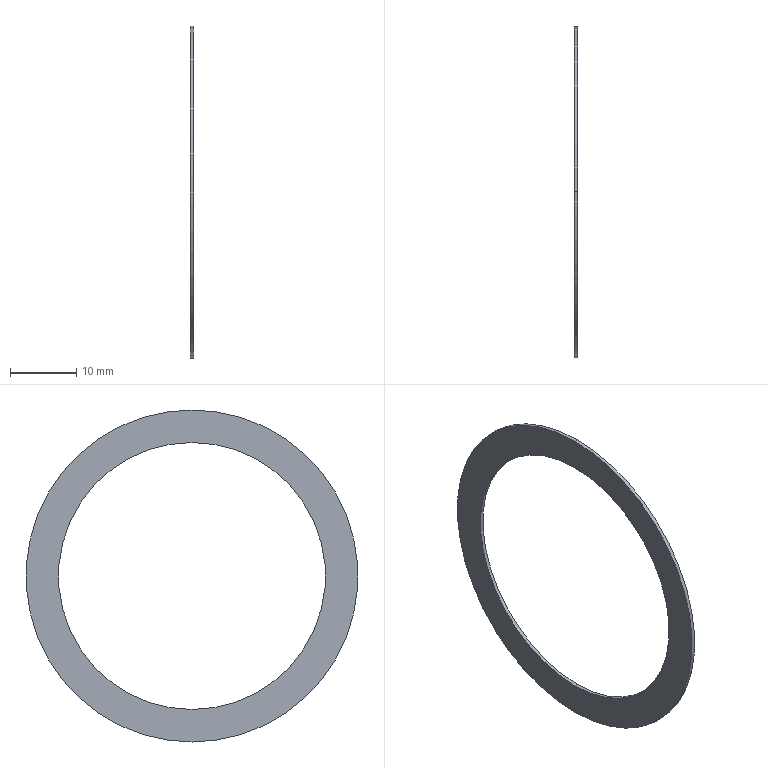Part | SolidWorks | features BaseBody 1 | 1 solid | 6 faces | box 0.54 x 50 x 50 mm | volume 374.901 mm3 | cylinder 4 | plane 2 | commonest cylinder face diameters 40.2 x2 50 x2
STEP:
#1=CARTESIAN_POINT('',(-9.68,63.,17.9));
#2=VERTEX_POINT('',#1);
#3=CARTESIAN_POINT('',(-9.68,63.,67.9));
#4=VERTEX_POINT('',#3);
#5=CARTESIAN_POINT('',(-9.68,63.,42.9));
#6=DIRECTION('',(1.,0.,0.));
#7=DIRECTION('',(0.,0.,-1.));
#8=AXIS2_PLACEMENT_3D('',#5,#6,#7);
#9=CIRCLE('',#8,25.);
#10=EDGE_CURVE('',#2,#4,#9,.T.);
#11=ORIENTED_EDGE('',*,*,#10,.T.);
#12=CARTESIAN_POINT('',(-9.14,63.,67.9));
#13=VERTEX_POINT('',#12);
#14=CARTESIAN_POINT('',(-9.41,63.,67.9));
#15=DIRECTION('',(1.,0.,0.));
#16=VECTOR('',#15,1000.);
#17=LINE('',#14,#16);
#18=EDGE_CURVE('',#4,#13,#17,.T.);
#19=ORIENTED_EDGE('',*,*,#18,.T.);
#20=CARTESIAN_POINT('',(-9.14,63.,17.9));
#21=VERTEX_POINT('',#20);
#22=CARTESIAN_POINT('',(-9.14,63.,42.9));
#23=DIRECTION('',(1.,0.,0.));
#24=DIRECTION('',(0.,0.,-1.));
#25=AXIS2_PLACEMENT_3D('',#22,#23,#24);
#26=CIRCLE('',#25,25.);
#27=EDGE_CURVE('',#21,#13,#26,.T.);
#28=ORIENTED_EDGE('',*,*,#27,.F.);
#29=CARTESIAN_POINT('',(-9.41,63.,17.9));
#30=DIRECTION('',(1.,0.,0.));
#31=VECTOR('',#30,1000.);
#32=LINE('',#29,#31);
#33=EDGE_CURVE('',#2,#21,#32,.T.);
#34=ORIENTED_EDGE('',*,*,#33,.F.);
#35=EDGE_LOOP('',(#11,#19,#28,#34));
#36=FACE_OUTER_BOUND('',#35,.T.);
#37=CARTESIAN_POINT('',(-9.41,63.,42.9));
#38=DIRECTION('',(1.,0.,0.));
#39=DIRECTION('',(0.,0.,-1.));
#40=AXIS2_PLACEMENT_3D('',#37,#38,#39);
#41=CYLINDRICAL_SURFACE('',#40,25.);
#42=ADVANCED_FACE('',(#36),#41,.T.);
#43=CARTESIAN_POINT('',(-9.68,63.,22.8));
#44=VERTEX_POINT('',#43);
#45=CARTESIAN_POINT('',(-9.68,63.,63.));
#46=VERTEX_POINT('',#45);
#47=CARTESIAN_POINT('',(-9.68,63.,42.9));
#48=DIRECTION('',(-1.,0.,0.));
#49=DIRECTION('',(0.,0.,-1.));
#50=AXIS2_PLACEMENT_3D('',#47,#48,#49);
#51=CIRCLE('',#50,20.1);
#52=EDGE_CURVE('',#44,#46,#51,.T.);
#53=ORIENTED_EDGE('',*,*,#52,.T.);
#54=CARTESIAN_POINT('',(-9.14,63.,63.));
#55=VERTEX_POINT('',#54);
#56=CARTESIAN_POINT('',(-9.68,63.,63.));
#57=DIRECTION('',(1.,0.,0.));
#58=VECTOR('',#57,1000.);
#59=LINE('',#56,#58);
#60=EDGE_CURVE('',#46,#55,#59,.T.);
#61=ORIENTED_EDGE('',*,*,#60,.T.);
#62=CARTESIAN_POINT('',(-9.14,63.,22.8));
#63=VERTEX_POINT('',#62);
#64=CARTESIAN_POINT('',(-9.14,63.,42.9));
#65=DIRECTION('',(-1.,0.,0.));
#66=DIRECTION('',(0.,0.,-1.));
#67=AXIS2_PLACEMENT_3D('',#64,#65,#66);
#68=CIRCLE('',#67,20.1);
#69=EDGE_CURVE('',#63,#55,#68,.T.);
#70=ORIENTED_EDGE('',*,*,#69,.F.);
#71=CARTESIAN_POINT('',(-9.68,63.,22.8));
#72=DIRECTION('',(1.,0.,0.));
#73=VECTOR('',#72,1000.);
#74=LINE('',#71,#73);
#75=EDGE_CURVE('',#44,#63,#74,.T.);
#76=ORIENTED_EDGE('',*,*,#75,.F.);
#77=EDGE_LOOP('',(#53,#61,#70,#76));
#78=FACE_OUTER_BOUND('',#77,.T.);
#79=CARTESIAN_POINT('',(-9.68,63.,42.9));
#80=DIRECTION('',(1.,0.,0.));
#81=DIRECTION('',(0.,0.,-1.));
#82=AXIS2_PLACEMENT_3D('',#79,#80,#81);
#83=CYLINDRICAL_SURFACE('',#82,20.1);
#84=ADVANCED_FACE('',(#78),#83,.F.);
#85=ORIENTED_EDGE('',*,*,#27,.T.);
#86=CARTESIAN_POINT('',(-9.14,63.,42.9));
#87=DIRECTION('',(1.,0.,0.));
#88=DIRECTION('',(0.,0.,-1.));
#89=AXIS2_PLACEMENT_3D('',#86,#87,#88);
#90=CIRCLE('',#89,25.);
#91=EDGE_CURVE('',#13,#21,#90,.T.);
#92=ORIENTED_EDGE('',*,*,#91,.T.);
#93=EDGE_LOOP('',(#85,#92));
#94=FACE_OUTER_BOUND('',#93,.T.);
#95=ORIENTED_EDGE('',*,*,#69,.T.);
#96=CARTESIAN_POINT('',(-9.14,63.,42.9));
#97=DIRECTION('',(-1.,0.,0.));
#98=DIRECTION('',(0.,0.,-1.));
#99=AXIS2_PLACEMENT_3D('',#96,#97,#98);
#100=CIRCLE('',#99,20.1);
#101=EDGE_CURVE('',#55,#63,#100,.T.);
#102=ORIENTED_EDGE('',*,*,#101,.T.);
#103=EDGE_LOOP('',(#95,#102));
#104=FACE_BOUND('',#103,.T.);
#105=CARTESIAN_POINT('',(-9.14,63.,65.45));
#106=DIRECTION('',(1.,0.,0.));
#107=DIRECTION('',(0.,0.,-1.));
#108=AXIS2_PLACEMENT_3D('',#105,#106,#107);
#109=PLANE('',#108);
#110=ADVANCED_FACE('',(#94,#104),#109,.T.);
#111=ORIENTED_EDGE('',*,*,#18,.F.);
#112=CARTESIAN_POINT('',(-9.68,63.,42.9));
#113=DIRECTION('',(1.,0.,0.));
#114=DIRECTION('',(0.,0.,-1.));
#115=AXIS2_PLACEMENT_3D('',#112,#113,#114);
#116=CIRCLE('',#115,25.);
#117=EDGE_CURVE('',#4,#2,#116,.T.);
#118=ORIENTED_EDGE('',*,*,#117,.T.);
#119=ORIENTED_EDGE('',*,*,#33,.T.);
#120=ORIENTED_EDGE('',*,*,#91,.F.);
#121=EDGE_LOOP('',(#111,#118,#119,#120));
#122=FACE_OUTER_BOUND('',#121,.T.);
#123=CARTESIAN_POINT('',(-9.41,63.,42.9));
#124=DIRECTION('',(1.,0.,0.));
#125=DIRECTION('',(0.,0.,-1.));
#126=AXIS2_PLACEMENT_3D('',#123,#124,#125);
#127=CYLINDRICAL_SURFACE('',#126,25.);
#128=ADVANCED_FACE('',(#122),#127,.T.);
#129=ORIENTED_EDGE('',*,*,#60,.F.);
#130=CARTESIAN_POINT('',(-9.68,63.,42.9));
#131=DIRECTION('',(-1.,0.,0.));
#132=DIRECTION('',(0.,0.,-1.));
#133=AXIS2_PLACEMENT_3D('',#130,#131,#132);
#134=CIRCLE('',#133,20.1);
#135=EDGE_CURVE('',#46,#44,#134,.T.);
#136=ORIENTED_EDGE('',*,*,#135,.T.);
#137=ORIENTED_EDGE('',*,*,#75,.T.);
#138=ORIENTED_EDGE('',*,*,#101,.F.);
#139=EDGE_LOOP('',(#129,#136,#137,#138));
#140=FACE_OUTER_BOUND('',#139,.T.);
#141=CARTESIAN_POINT('',(-9.68,63.,42.9));
#142=DIRECTION('',(1.,0.,0.));
#143=DIRECTION('',(0.,0.,-1.));
#144=AXIS2_PLACEMENT_3D('',#141,#142,#143);
#145=CYLINDRICAL_SURFACE('',#144,20.1);
#146=ADVANCED_FACE('',(#140),#145,.F.);
#147=ORIENTED_EDGE('',*,*,#52,.F.);
#148=ORIENTED_EDGE('',*,*,#135,.F.);
#149=EDGE_LOOP('',(#147,#148));
#150=FACE_BOUND('',#149,.T.);
#151=ORIENTED_EDGE('',*,*,#10,.F.);
#152=ORIENTED_EDGE('',*,*,#117,.F.);
#153=EDGE_LOOP('',(#151,#152));
#154=FACE_OUTER_BOUND('',#153,.T.);
#155=CARTESIAN_POINT('',(-9.68,63.,65.45));
#156=DIRECTION('',(-1.,0.,0.));
#157=DIRECTION('',(0.,0.,1.));
#158=AXIS2_PLACEMENT_3D('',#155,#156,#157);
#159=PLANE('',#158);
#160=ADVANCED_FACE('',(#150,#154),#159,.T.);
#161=CLOSED_SHELL('',(#42,#84,#110,#128,#146,#160));
#162=MANIFOLD_SOLID_BREP('',#161);
#163=CARTESIAN_POINT('',(0.,0.,0.));
#164=DIRECTION('',(0.,0.,1.));
#165=DIRECTION('',(1.,0.,0.));
#166=AXIS2_PLACEMENT_3D('',#163,#164,#165);
#167=(LENGTH_UNIT()NAMED_UNIT(*)SI_UNIT(.MILLI.,.METRE.));
#168=UNCERTAINTY_MEASURE_WITH_UNIT(LENGTH_MEASURE(0.00001),#167,'','');
#169=(NAMED_UNIT(*)PLANE_ANGLE_UNIT()SI_UNIT($,.RADIAN.));
#170=(NAMED_UNIT(*)SI_UNIT($,.STERADIAN.)SOLID_ANGLE_UNIT());
#171=(GEOMETRIC_REPRESENTATION_CONTEXT(3)GLOBAL_UNCERTAINTY_ASSIGNED_CONTEXT((#168))GLOBAL_UNIT_ASSIGNED_CONTEXT((#167,#169,#170))REPRESENTATION_CONTEXT('',''));
#172=ADVANCED_BREP_SHAPE_REPRESENTATION('',(#162,#166),#171);